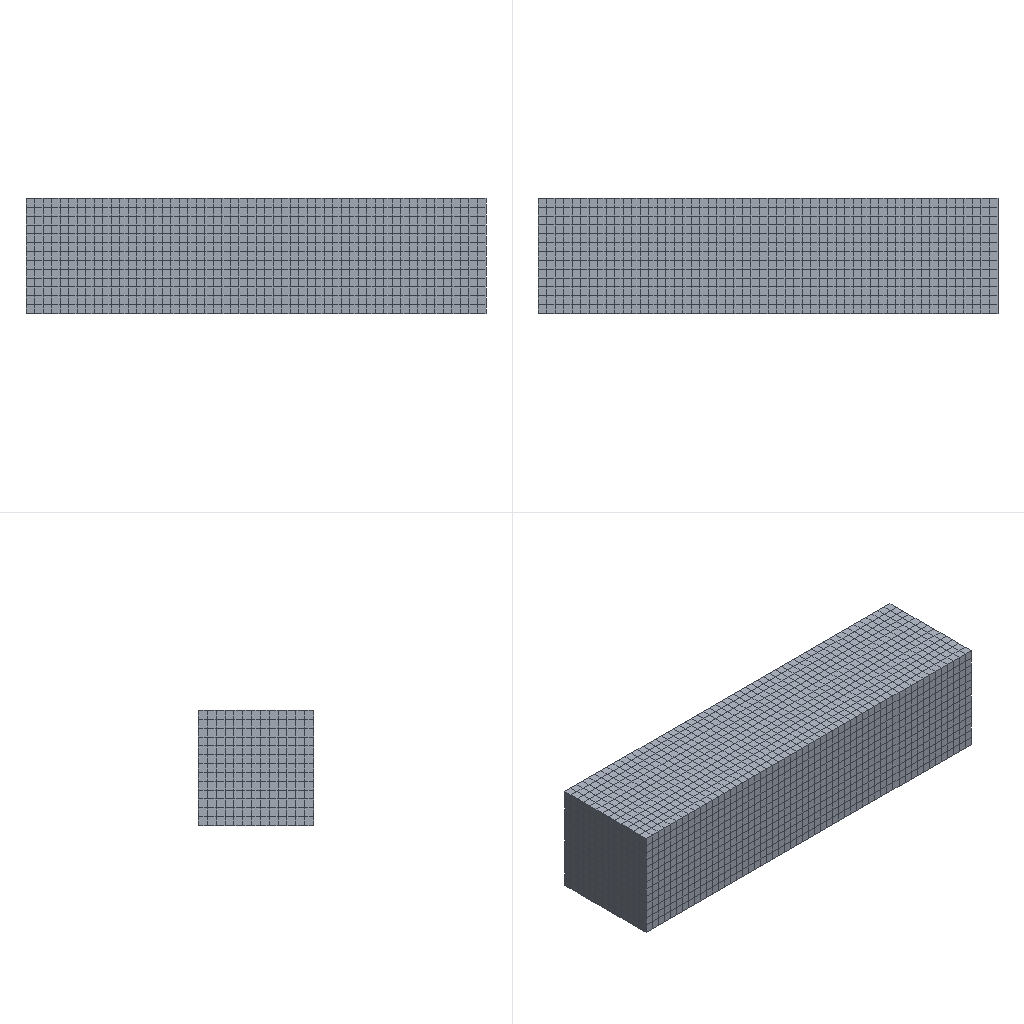Simulation study | abaqus
Set-up summary:
category,name,step,type,value,unit,region
solver,abaqus
solver,version,,,Abaqus/Standard 2020
units,not stated in the deck,,not stated
analysis,deck,,static,static
load_step,Step-1,Step-1,static
load_step,requested,,,1
mesh,nodes,,,19146
mesh,elements,,,15715
element_type,C3D8R,,solid,15546
element_type,COH3D8,,cohesive,169
load,load commands in deck,,count,1
bc,support commands in deck,,count,7
material,COH,,in results
material,JITI,,in results
material,XIANWEI,,in results
check,setup vs results,,match,"per instance, exact: element labels, types and connectivity; labels of the nodes the elements use; coordinates of those nodes at SINGLE_PRECISION in 1 of 2 instance(s)"
Abaqus input file, long lists of numbers shortened:
*Heading
** Job name: Job-1 Model name: Model-1
** Generated by: Abaqus/CAE 2020
*Preprint, echo=NO, model=NO, history=NO, contact=NO
**
** PARTS
**
*Part, name=jiti
*Node
      1,           4.,           0.,           0.
      2,           4.,           0.,           2.
** (10974 more lines like these left out)
*Element, type=C3D8R
   1, 10781, 10782,  3293,   989, 10784, 10783,   365,    88
   2, 10782, 10785,  3294,  3293, 10783, 10786,   366,   365
** (9124 more lines like these left out)
*Element, type=COH3D8
9127,     1,    13,  1613,   188, 10784, 10783, 10782, 10781
9128,    13,    14,  1614,  1613, 10783, 10786, 10785, 10782
** (167 more lines like these left out)
*Nset, nset=Set-6, generate
     1,  10976,      1
*Elset, elset=Set-6, generate
    1,  9126,     1
*Elset, elset=CohesiveSeam-1-Elements, generate
 9127,  9295,     1
*Nset, nset=CohesiveSeam-1-TopNodes, generate
 10781,  10976,      1
*Nset, nset=CohesiveSeam-1-BottomNodes
    1,    2,    5,    8,   13,   14,   15,   16,   17,   18,   19,   20,   21,   22,   23,   24
   89,   90,   91,   92,   93,   94,   95,   96,   97,   98,   99,  100,  177,  178,  179,  180
** (11 more lines like these left out)
*Elset, elset=__PickedSurf4_S2, internal, generate
 9127,  9295,     1
*Surface, type=ELEMENT, name=_PickedSurf4, internal
__PickedSurf4_S2, S2
*Elset, elset=_CohesiveSeam-1-TopSurf_S2, internal, generate
 9127,  9295,     1
*Surface, type=ELEMENT, name=CohesiveSeam-1-TopSurf
_CohesiveSeam-1-TopSurf_S2, S2
*Elset, elset=_CohesiveSeam-1-BottomSurf_S1, internal, generate
 9127,  9295,     1
*Surface, type=ELEMENT, name=CohesiveSeam-1-BottomSurf
_CohesiveSeam-1-BottomSurf_S1, S1
** Section: jiti
*Solid Section, elset=Set-6, material=jiti
,
** Section: coh
*Cohesive Section, elset=CohesiveSeam-1-Elements, controls=EC-1, material=coh, response=TRACTION SEPARATION
,
*End Part
**
*Part, name=xianwei
*Node
      1, -0.1368, -0.246,   7.126
      2, -0.1652,  -0.3277,    7.227
** (8168 more lines like these left out)
*Element, type=C3D8R
   1,   53,   39,   52,   63,   15,    1,   14,   25
   2,   54,   51,   50,   55,   16,   13,   12,   17
** (6418 more lines like these left out)
*Nset, nset=Set-1, generate
    1,  8170,     1
*Elset, elset=Set-1, generate
    1,  6420,     1
*Orientation, name=Ori-1
1., 0., 0., 0., 1., 0.
1, 0.
** Section: xianwei
*Solid Section, elset=Set-1, orientation=Ori-1, material=xianwei
,
*End Part
**
**
** ASSEMBLY
**
*Assembly, name=Assembly
**
*Instance, name=jiti-1, part=jiti
*End Instance
**
*Instance, name=xianwei-1, part=xianwei
         0.5,          -1.,           1.
         0.5,          -1.,           1.,          0.5, 1.26880521644779e-08,           1., 90.
*End Instance
**
*Node
      1,           8.,          -1.,           1.
*Nset, nset=Set-1, instance=jiti-1
    9,   10,   11,   12,  213,  214,  215,  216,  217,  218,  219,  220,  221,  222,  223,  224
  225,  226,  227,  228,  229,  230,  231,  232,  233,  234,  235,  236,  237,  238,  239,  240
** (11 more lines like these left out)
*Elset, elset=Set-1, instance=jiti-1, generate
 4564,  4732,     1
*Nset, nset=Set-3
 1,
*Nset, nset=Set-6, instance=jiti-1
     1,     4,     7,     8,    11,    12,    63,    64,    65,    66,    67,    68,    69,    70,    71,    72
    73,    74,    75,    76,    77,    78,    79,    80,    81,    82,    83,    84,    85,    86,    87,    88
** (47 more lines like these left out)
*Elset, elset=Set-6, instance=jiti-1
    1,   14,   27,   40,   53,   66,   79,   92,  105,  118,  131,  144,  157,  170,  183,  196
  209,  222,  235,  248,  261,  274,  287,  300,  313,  326,  339,  352,  365,  378,  391,  404
** (42 more lines like these left out)
*Nset, nset=Set-9, instance=jiti-1, generate
 1757,  1900,     1
*Elset, elset=Set-9, instance=jiti-1
  339,  340,  341,  342,  343,  344,  345,  346,  347,  348,  349,  350,  351,  690,  691,  692
  693,  694,  695,  696,  697,  698,  699,  700,  701,  702, 1041, 1042, 1043, 1044, 1045, 1046
** (9 more lines like these left out)
*Nset, nset=Set-10, instance=jiti-1
    3,    4,    6,    7,   51,   52,   53,   54,   55,   56,   57,   58,   59,   60,   61,   62
  127,  128,  129,  130,  131,  132,  133,  134,  135,  136,  137,  138,  165,  166,  167,  168
** (11 more lines like these left out)
*Elset, elset=Set-10, instance=jiti-1
  339,  340,  341,  342,  343,  344,  345,  346,  347,  348,  349,  350,  351,  690,  691,  692
  693,  694,  695,  696,  697,  698,  699,  700,  701,  702, 1041, 1042, 1043, 1044, 1045, 1046
** (9 more lines like these left out)
*Nset, nset=Set-11
 1,
*Nset, nset=m_Set-2
 1,
*Nset, nset=m_Set-4, instance=xianwei-1, generate
    1,  8170,     1
*Elset, elset=m_Set-4, instance=xianwei-1, generate
    1,  6420,     1
*Nset, nset=m_Set-7, instance=xianwei-1, generate
    1,  8170,     1
*Elset, elset=m_Set-7, instance=xianwei-1, generate
    1,  6420,     1
*Nset, nset=s_Set-4, instance=jiti-1, generate
     1,  10976,      1
*Elset, elset=s_Set-4, instance=jiti-1, generate
    1,  9126,     1
*Nset, nset=s_Set-7, instance=jiti-1, generate
     1,  10976,      1
*Elset, elset=s_Set-7, instance=jiti-1, generate
    1,  9126,     1
*Elset, elset=_s_Surf-1_S5, internal, instance=jiti-1
  339,  340,  341,  342,  343,  344,  345,  346,  347,  348,  349,  350,  351,  690,  691,  692
  693,  694,  695,  696,  697,  698,  699,  700,  701,  702, 1041, 1042, 1043, 1044, 1045, 1046
** (9 more lines like these left out)
*Surface, type=ELEMENT, name=s_Surf-1
_s_Surf-1_S5, S5
** Constraint: Constraint-1
*Coupling, constraint name=Constraint-1, ref node=m_Set-2, surface=s_Surf-1
*Kinematic
** Constraint: Constraint-2
*Embedded Element, host elset=s_Set-7
m_Set-7
*End Assembly
**
** ELEMENT CONTROLS
**
*Section Controls, name=EC-1, ELEMENT DELETION=YES
1., 1., 1.
*Amplitude, name=Amp-1
             0.,              0.,              1.,              1.
**
** MATERIALS
**
*Material, name=coh
*Damage Initiation, criterion=MAXS
1.,1.,1.
*Damage Evolution, type=DISPLACEMENT
 1e-18,
*Elastic, type=TRACTION
20.,20.,20.
*Material, name=jiti
*Elastic
20., 0.45
*Material, name=xianwei
*Elastic
300., 0.4
*Fail Stress
1.,  1.,  1.,  1.,120.,  0.,150.
** ----------------------------------------------------------------
**
** STEP: Step-1
**
*Step, name=Step-1, nlgeom=YES, inc=10000
*Static, stabilize=0.0002, allsdtol=0.05, continue=NO
0.01, 1., 1e-08, 1.
**
** BOUNDARY CONDITIONS
**
** Name: BC-1 Type: 对称/反对称/完全固定
*Boundary
Set-1, ENCASTRE
** Name: BC-2 Type: 位移/转角
*Boundary, amplitude=Amp-1
Set-11, 1, 1, 20.
Set-11, 2, 2
Set-11, 3, 3
Set-11, 4, 4
Set-11, 5, 5
Set-11, 6, 6
**
** CONTROLS
**
*Controls, reset
*Controls, parameters=time incrementation
, , , , , , , 20, , ,
**
** OUTPUT REQUESTS
**
*Restart, write, number interval=1, time marks=NO
**
** FIELD OUTPUT: F-Output-1
**
*Output, field
*Node Output
CF, PHILSM, PSILSM, RF, RM, RT, U, V
*Element Output, directions=YES
CFAILURE, DAMAGEC, DAMAGEFC, DAMAGEFT, DAMAGEMC, DAMAGEMT, DAMAGESHR, DAMAGET, DMICRT, E, ENRRTXFEM, ERPRATIO, HSNFCCRT, HSNFTCRT, HSNMCCRT, HSNMTCRT
JK, LE, MISES, MISESMAX, MISESONLY, PE, PEEQ, PEMAG, S, SDEG, SHRRATIO, SSAVG, STATUS, YIELDPOT
*Contact Output
BDSTAT, CDISP, CRSTS, CSDMG, CSMAXSCRT, CSMAXUCRT, CSQUADSCRT, CSQUADUCRT, CSTRESS, DBS, DBSF, DBT, EFENRRTR, ENRRT, OPENBC
**
** HISTORY OUTPUT: H-Output-1
**
*Output, history
*Node Output, nset=Set-11
RF1, U1
*End Step
Results summary:
result,step,,partial,increments=332 time=0.03602/1.0
result,analysis,,,static
result,last_loadstep,,,1
result,primary field,,,U
result,reaction total,,FX,0.3514,model units
result,reaction total,,FY,-0.004648,model units
result,reaction total,,FZ,0.02317,model units